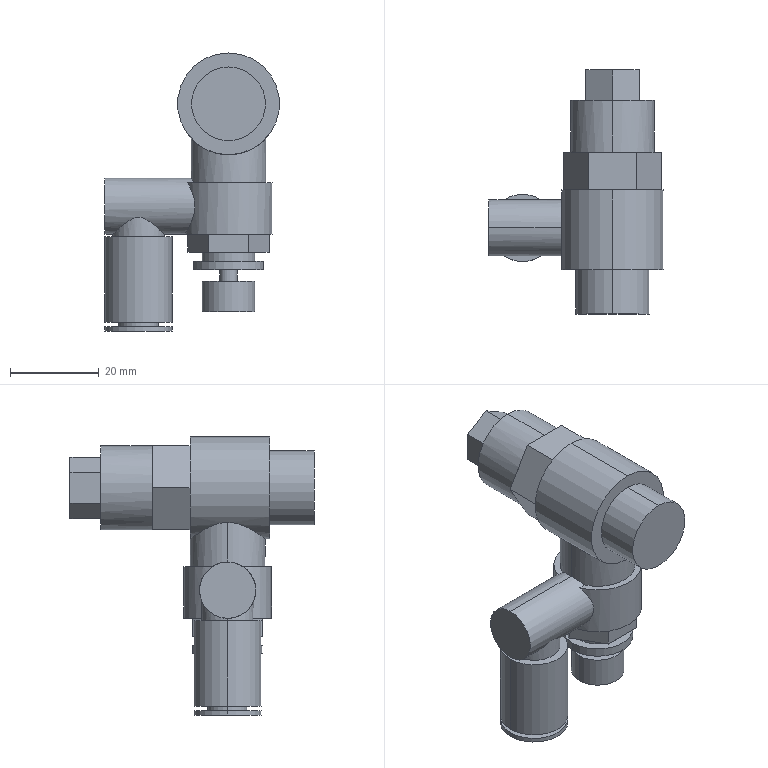Part | STEP file | Speed control valve with pilot-operated air lock ASP530F-03-08S | 1 solid | 76 faces | box 39.4 x 55.1 x 62.8 mm | volume 28936 mm3 | plane 43 | cylinder 31 | cone 2 | commonest cylinder face diameters 11.88 x4 15.2 x4 4 x2 8 x2 8.566 x2 9 x2